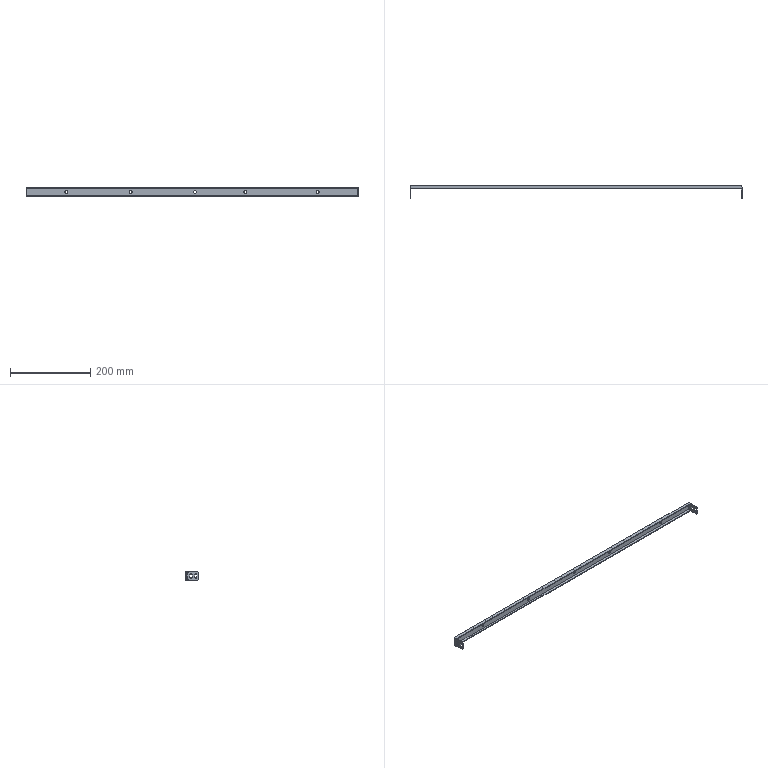Part | SolidWorks | features ICE 3, Chamfer 1, Extrusion 1, Fillet 1, HoleWzd 1 | 1 solid | 50 faces | box 825 x 30 x 22 mm | volume 48151 mm3 | plane 26 | cylinder 24 | commonest cylinder face diameters 5 x12 7 x10 6 x2